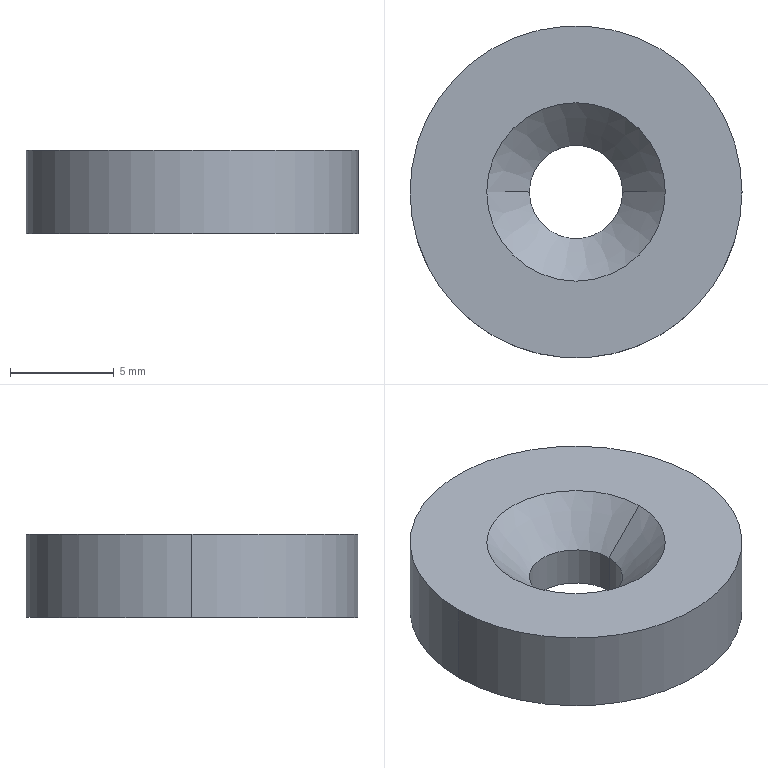Part | STEP file | Screen clamp adjusting cap | 1 solid | 8 faces | box 16 x 16 x 4 mm | volume 701.903 mm3 | cylinder 4 | cone 2 | plane 2 | commonest cylinder face diameters 4.5 x2 16 x2
STEP:
#1=CARTESIAN_POINT('',(-2.25,0.,1.95));
#2=VERTEX_POINT('',#1);
#3=CARTESIAN_POINT('',(2.25,0.,1.95));
#4=VERTEX_POINT('',#3);
#5=CARTESIAN_POINT('',(0.,0.,1.95));
#6=DIRECTION('',(0.,0.,1.));
#7=DIRECTION('',(1.,0.,0.));
#8=AXIS2_PLACEMENT_3D('',#5,#6,#7);
#9=CIRCLE('',#8,2.25);
#10=EDGE_CURVE('',#2,#4,#9,.T.);
#11=ORIENTED_EDGE('',*,*,#10,.F.);
#12=CARTESIAN_POINT('',(-4.3,0.,4.));
#13=VERTEX_POINT('',#12);
#14=CARTESIAN_POINT('',(-4.3,0.,4.));
#15=DIRECTION('',(-0.7071,0.,0.7071));
#16=VECTOR('',#15,1000.);
#17=LINE('',#14,#16);
#18=EDGE_CURVE('',#2,#13,#17,.T.);
#19=ORIENTED_EDGE('',*,*,#18,.T.);
#20=CARTESIAN_POINT('',(4.3,0.,4.));
#21=VERTEX_POINT('',#20);
#22=CARTESIAN_POINT('',(0.,0.,4.));
#23=DIRECTION('',(0.,0.,1.));
#24=DIRECTION('',(1.,0.,0.));
#25=AXIS2_PLACEMENT_3D('',#22,#23,#24);
#26=CIRCLE('',#25,4.3);
#27=EDGE_CURVE('',#13,#21,#26,.T.);
#28=ORIENTED_EDGE('',*,*,#27,.T.);
#29=CARTESIAN_POINT('',(4.3,0.,4.));
#30=DIRECTION('',(0.7071,0.,0.7071));
#31=VECTOR('',#30,1000.);
#32=LINE('',#29,#31);
#33=EDGE_CURVE('',#4,#21,#32,.T.);
#34=ORIENTED_EDGE('',*,*,#33,.F.);
#35=EDGE_LOOP('',(#11,#19,#28,#34));
#36=FACE_OUTER_BOUND('',#35,.T.);
#37=CARTESIAN_POINT('',(0.,0.,4.));
#38=DIRECTION('',(0.,0.,1.));
#39=DIRECTION('',(1.,0.,0.));
#40=AXIS2_PLACEMENT_3D('',#37,#38,#39);
#41=CONICAL_SURFACE('',#40,4.3,0.7854);
#42=ADVANCED_FACE('',(#36),#41,.F.);
#43=CARTESIAN_POINT('',(-2.25,0.,0.));
#44=VERTEX_POINT('',#43);
#45=CARTESIAN_POINT('',(2.25,0.,0.));
#46=VERTEX_POINT('',#45);
#47=CARTESIAN_POINT('',(0.,0.,0.));
#48=DIRECTION('',(0.,0.,1.));
#49=DIRECTION('',(1.,0.,0.));
#50=AXIS2_PLACEMENT_3D('',#47,#48,#49);
#51=CIRCLE('',#50,2.25);
#52=EDGE_CURVE('',#44,#46,#51,.T.);
#53=ORIENTED_EDGE('',*,*,#52,.F.);
#54=CARTESIAN_POINT('',(-2.25,0.,4.));
#55=DIRECTION('',(0.,0.,1.));
#56=VECTOR('',#55,1000.);
#57=LINE('',#54,#56);
#58=EDGE_CURVE('',#44,#2,#57,.T.);
#59=ORIENTED_EDGE('',*,*,#58,.T.);
#60=ORIENTED_EDGE('',*,*,#10,.T.);
#61=CARTESIAN_POINT('',(2.25,0.,4.));
#62=DIRECTION('',(0.,0.,1.));
#63=VECTOR('',#62,1000.);
#64=LINE('',#61,#63);
#65=EDGE_CURVE('',#46,#4,#64,.T.);
#66=ORIENTED_EDGE('',*,*,#65,.F.);
#67=EDGE_LOOP('',(#53,#59,#60,#66));
#68=FACE_OUTER_BOUND('',#67,.T.);
#69=CARTESIAN_POINT('',(0.,0.,4.));
#70=DIRECTION('',(0.,0.,1.));
#71=DIRECTION('',(1.,0.,0.));
#72=AXIS2_PLACEMENT_3D('',#69,#70,#71);
#73=CYLINDRICAL_SURFACE('',#72,2.25);
#74=ADVANCED_FACE('',(#68),#73,.F.);
#75=CARTESIAN_POINT('',(8.,0.,4.));
#76=VERTEX_POINT('',#75);
#77=CARTESIAN_POINT('',(-8.,0.,4.));
#78=VERTEX_POINT('',#77);
#79=CARTESIAN_POINT('',(0.,0.,4.));
#80=DIRECTION('',(0.,0.,1.));
#81=DIRECTION('',(1.,0.,0.));
#82=AXIS2_PLACEMENT_3D('',#79,#80,#81);
#83=CIRCLE('',#82,8.);
#84=EDGE_CURVE('',#76,#78,#83,.T.);
#85=ORIENTED_EDGE('',*,*,#84,.F.);
#86=CARTESIAN_POINT('',(8.,0.,0.));
#87=VERTEX_POINT('',#86);
#88=CARTESIAN_POINT('',(8.,0.,4.));
#89=DIRECTION('',(0.,0.,-1.));
#90=VECTOR('',#89,1000.);
#91=LINE('',#88,#90);
#92=EDGE_CURVE('',#76,#87,#91,.T.);
#93=ORIENTED_EDGE('',*,*,#92,.T.);
#94=CARTESIAN_POINT('',(-8.,0.,0.));
#95=VERTEX_POINT('',#94);
#96=CARTESIAN_POINT('',(0.,0.,0.));
#97=DIRECTION('',(0.,0.,1.));
#98=DIRECTION('',(1.,0.,0.));
#99=AXIS2_PLACEMENT_3D('',#96,#97,#98);
#100=CIRCLE('',#99,8.);
#101=EDGE_CURVE('',#87,#95,#100,.T.);
#102=ORIENTED_EDGE('',*,*,#101,.T.);
#103=CARTESIAN_POINT('',(-8.,0.,4.));
#104=DIRECTION('',(0.,0.,-1.));
#105=VECTOR('',#104,1000.);
#106=LINE('',#103,#105);
#107=EDGE_CURVE('',#78,#95,#106,.T.);
#108=ORIENTED_EDGE('',*,*,#107,.F.);
#109=EDGE_LOOP('',(#85,#93,#102,#108));
#110=FACE_OUTER_BOUND('',#109,.T.);
#111=CARTESIAN_POINT('',(0.,0.,4.));
#112=DIRECTION('',(0.,0.,-1.));
#113=DIRECTION('',(-1.,0.,0.));
#114=AXIS2_PLACEMENT_3D('',#111,#112,#113);
#115=CYLINDRICAL_SURFACE('',#114,8.);
#116=ADVANCED_FACE('',(#110),#115,.T.);
#117=ORIENTED_EDGE('',*,*,#92,.F.);
#118=CARTESIAN_POINT('',(0.,0.,4.));
#119=DIRECTION('',(0.,0.,1.));
#120=DIRECTION('',(1.,0.,0.));
#121=AXIS2_PLACEMENT_3D('',#118,#119,#120);
#122=CIRCLE('',#121,8.);
#123=EDGE_CURVE('',#78,#76,#122,.T.);
#124=ORIENTED_EDGE('',*,*,#123,.F.);
#125=ORIENTED_EDGE('',*,*,#107,.T.);
#126=CARTESIAN_POINT('',(0.,0.,0.));
#127=DIRECTION('',(0.,0.,1.));
#128=DIRECTION('',(1.,0.,0.));
#129=AXIS2_PLACEMENT_3D('',#126,#127,#128);
#130=CIRCLE('',#129,8.);
#131=EDGE_CURVE('',#95,#87,#130,.T.);
#132=ORIENTED_EDGE('',*,*,#131,.T.);
#133=EDGE_LOOP('',(#117,#124,#125,#132));
#134=FACE_OUTER_BOUND('',#133,.T.);
#135=CARTESIAN_POINT('',(0.,0.,4.));
#136=DIRECTION('',(0.,0.,-1.));
#137=DIRECTION('',(-1.,0.,0.));
#138=AXIS2_PLACEMENT_3D('',#135,#136,#137);
#139=CYLINDRICAL_SURFACE('',#138,8.);
#140=ADVANCED_FACE('',(#134),#139,.T.);
#141=CARTESIAN_POINT('',(0.,0.,4.));
#142=DIRECTION('',(0.,0.,1.));
#143=DIRECTION('',(1.,0.,0.));
#144=AXIS2_PLACEMENT_3D('',#141,#142,#143);
#145=CIRCLE('',#144,4.3);
#146=EDGE_CURVE('',#21,#13,#145,.T.);
#147=ORIENTED_EDGE('',*,*,#146,.F.);
#148=ORIENTED_EDGE('',*,*,#27,.F.);
#149=EDGE_LOOP('',(#147,#148));
#150=FACE_BOUND('',#149,.T.);
#151=ORIENTED_EDGE('',*,*,#123,.T.);
#152=ORIENTED_EDGE('',*,*,#84,.T.);
#153=EDGE_LOOP('',(#151,#152));
#154=FACE_OUTER_BOUND('',#153,.T.);
#155=CARTESIAN_POINT('',(0.,0.,4.));
#156=DIRECTION('',(0.,0.,1.));
#157=DIRECTION('',(1.,0.,0.));
#158=AXIS2_PLACEMENT_3D('',#155,#156,#157);
#159=PLANE('',#158);
#160=ADVANCED_FACE('',(#150,#154),#159,.T.);
#161=CARTESIAN_POINT('',(0.,0.,0.));
#162=DIRECTION('',(0.,0.,1.));
#163=DIRECTION('',(1.,0.,0.));
#164=AXIS2_PLACEMENT_3D('',#161,#162,#163);
#165=CIRCLE('',#164,2.25);
#166=EDGE_CURVE('',#46,#44,#165,.T.);
#167=ORIENTED_EDGE('',*,*,#166,.T.);
#168=ORIENTED_EDGE('',*,*,#52,.T.);
#169=EDGE_LOOP('',(#167,#168));
#170=FACE_BOUND('',#169,.T.);
#171=ORIENTED_EDGE('',*,*,#131,.F.);
#172=ORIENTED_EDGE('',*,*,#101,.F.);
#173=EDGE_LOOP('',(#171,#172));
#174=FACE_OUTER_BOUND('',#173,.T.);
#175=CARTESIAN_POINT('',(0.,0.,0.));
#176=DIRECTION('',(0.,0.,1.));
#177=DIRECTION('',(1.,0.,0.));
#178=AXIS2_PLACEMENT_3D('',#175,#176,#177);
#179=PLANE('',#178);
#180=ADVANCED_FACE('',(#170,#174),#179,.F.);
#181=ORIENTED_EDGE('',*,*,#58,.F.);
#182=ORIENTED_EDGE('',*,*,#166,.F.);
#183=ORIENTED_EDGE('',*,*,#65,.T.);
#184=CARTESIAN_POINT('',(0.,0.,1.95));
#185=DIRECTION('',(0.,0.,1.));
#186=DIRECTION('',(1.,0.,0.));
#187=AXIS2_PLACEMENT_3D('',#184,#185,#186);
#188=CIRCLE('',#187,2.25);
#189=EDGE_CURVE('',#4,#2,#188,.T.);
#190=ORIENTED_EDGE('',*,*,#189,.T.);
#191=EDGE_LOOP('',(#181,#182,#183,#190));
#192=FACE_OUTER_BOUND('',#191,.T.);
#193=CARTESIAN_POINT('',(0.,0.,4.));
#194=DIRECTION('',(0.,0.,1.));
#195=DIRECTION('',(1.,0.,0.));
#196=AXIS2_PLACEMENT_3D('',#193,#194,#195);
#197=CYLINDRICAL_SURFACE('',#196,2.25);
#198=ADVANCED_FACE('',(#192),#197,.F.);
#199=ORIENTED_EDGE('',*,*,#18,.F.);
#200=ORIENTED_EDGE('',*,*,#189,.F.);
#201=ORIENTED_EDGE('',*,*,#33,.T.);
#202=ORIENTED_EDGE('',*,*,#146,.T.);
#203=EDGE_LOOP('',(#199,#200,#201,#202));
#204=FACE_OUTER_BOUND('',#203,.T.);
#205=CARTESIAN_POINT('',(0.,0.,4.));
#206=DIRECTION('',(0.,0.,1.));
#207=DIRECTION('',(1.,0.,0.));
#208=AXIS2_PLACEMENT_3D('',#205,#206,#207);
#209=CONICAL_SURFACE('',#208,4.3,0.7854);
#210=ADVANCED_FACE('',(#204),#209,.F.);
#211=CLOSED_SHELL('',(#42,#74,#116,#140,#160,#180,#198,#210));
#212=MANIFOLD_SOLID_BREP('',#211);
#213=CARTESIAN_POINT('',(0.,0.,0.));
#214=DIRECTION('',(0.,0.,1.));
#215=DIRECTION('',(1.,0.,0.));
#216=AXIS2_PLACEMENT_3D('',#213,#214,#215);
#217=(LENGTH_UNIT()NAMED_UNIT(*)SI_UNIT(.MILLI.,.METRE.));
#218=UNCERTAINTY_MEASURE_WITH_UNIT(LENGTH_MEASURE(0.00001),#217,'','');
#219=(NAMED_UNIT(*)PLANE_ANGLE_UNIT()SI_UNIT($,.RADIAN.));
#220=(NAMED_UNIT(*)SI_UNIT($,.STERADIAN.)SOLID_ANGLE_UNIT());
#221=(GEOMETRIC_REPRESENTATION_CONTEXT(3)GLOBAL_UNCERTAINTY_ASSIGNED_CONTEXT((#218))GLOBAL_UNIT_ASSIGNED_CONTEXT((#217,#219,#220))REPRESENTATION_CONTEXT('',''));
#222=ADVANCED_BREP_SHAPE_REPRESENTATION('',(#212,#216),#221);